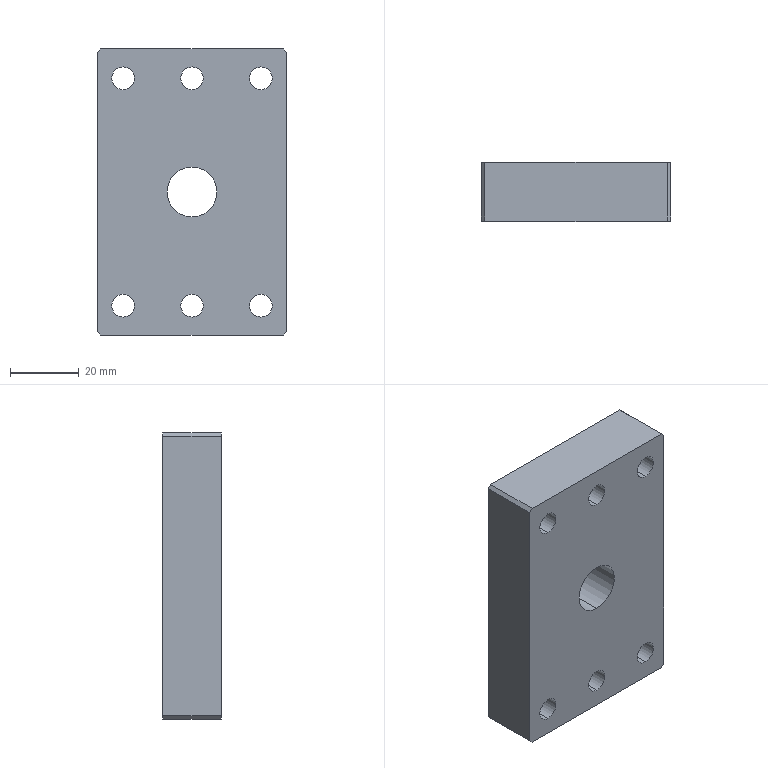Part | STEP file | 1 solid | 42 faces | box 55 x 17 x 83 mm | volume 68793 mm3 | cylinder 26 | plane 16 | commonest cylinder face diameters 6.6 x12 11 x12 14.5 x2